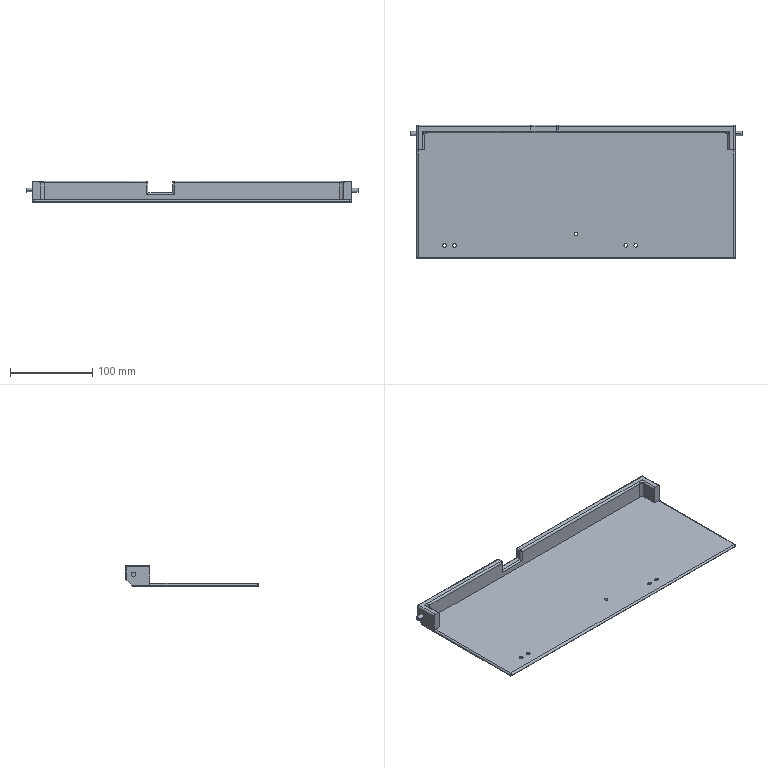Part | STEP file | 11-FG99-2015-7-17-S010-V3.0-kkkkkk-998.11 | 1 solid | 81 faces | box 403 x 162 x 26 mm | volume 310656 mm3 | cylinder 40 | plane 19 | sphere 10 | cone 8 | spline 4 | commonest cylinder face diameters 4 x24 4.5 x8 5 x4 4.2 x2 10 x2